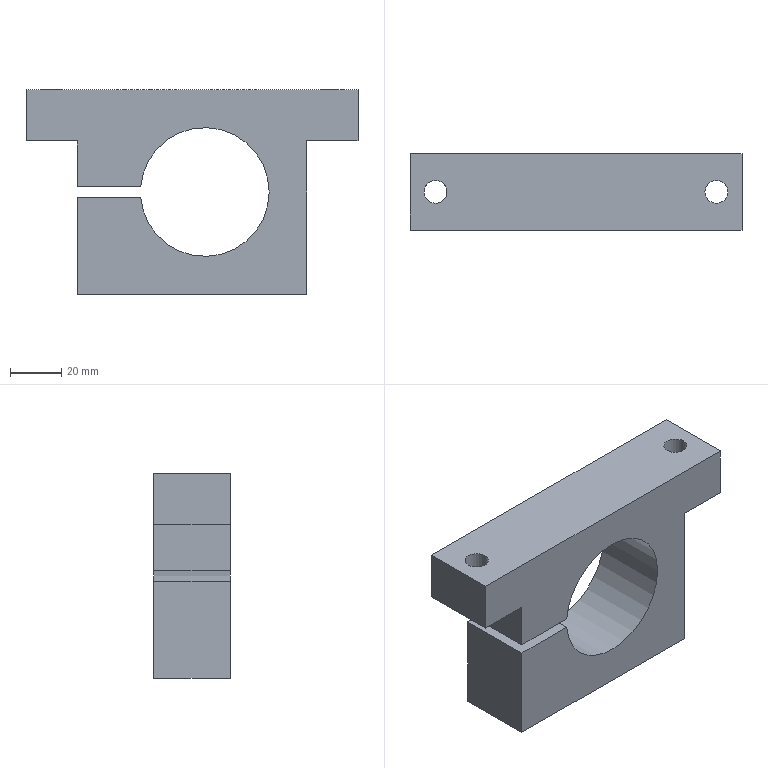Part | NX | features MAIN_BODY 2 | 1 solid | 16 faces | box 130 x 30 x 80 mm | volume 174625 mm3 | plane 13 | cylinder 3 | commonest cylinder face diameters 9 x2 50.4 x1
STEP:
#1=CARTESIAN_POINT('',(-547.,-675.001,150.));
#2=VERTEX_POINT('',#1);
#3=CARTESIAN_POINT('',(-547.,-675.001,170.));
#4=VERTEX_POINT('',#3);
#5=CARTESIAN_POINT('',(-547.,-675.001,150.));
#6=DIRECTION('',(0.,0.,1.));
#7=VECTOR('',#6,1000.);
#8=LINE('',#5,#7);
#9=EDGE_CURVE('',#2,#4,#8,.T.);
#10=ORIENTED_EDGE('',*,*,#9,.F.);
#11=CARTESIAN_POINT('',(-547.,-705.001,150.));
#12=VERTEX_POINT('',#11);
#13=CARTESIAN_POINT('',(-547.,-705.001,150.));
#14=DIRECTION('',(0.,1.,0.));
#15=VECTOR('',#14,1000.);
#16=LINE('',#13,#15);
#17=EDGE_CURVE('',#12,#2,#16,.T.);
#18=ORIENTED_EDGE('',*,*,#17,.F.);
#19=CARTESIAN_POINT('',(-547.,-705.001,170.));
#20=VERTEX_POINT('',#19);
#21=CARTESIAN_POINT('',(-547.,-705.001,150.));
#22=DIRECTION('',(0.,0.,1.));
#23=VECTOR('',#22,1000.);
#24=LINE('',#21,#23);
#25=EDGE_CURVE('',#12,#20,#24,.T.);
#26=ORIENTED_EDGE('',*,*,#25,.T.);
#27=CARTESIAN_POINT('',(-547.,-705.001,170.));
#28=DIRECTION('',(0.,1.,0.));
#29=VECTOR('',#28,1000.);
#30=LINE('',#27,#29);
#31=EDGE_CURVE('',#20,#4,#30,.T.);
#32=ORIENTED_EDGE('',*,*,#31,.T.);
#33=EDGE_LOOP('',(#10,#18,#26,#32));
#34=FACE_BOUND('',#33,.T.);
#35=CARTESIAN_POINT('',(-547.,-705.001,150.));
#36=DIRECTION('',(-1.,0.,0.));
#37=DIRECTION('',(0.,1.,0.));
#38=AXIS2_PLACEMENT_3D('',#35,#36,#37);
#39=PLANE('',#38);
#40=ADVANCED_FACE('',(#34),#39,.T.);
#41=CARTESIAN_POINT('',(-431.5,-690.001,170.));
#42=VERTEX_POINT('',#41);
#43=CARTESIAN_POINT('',(-427.,-690.001,170.));
#44=DIRECTION('',(0.,0.,1.));
#45=DIRECTION('',(-1.,0.,0.));
#46=AXIS2_PLACEMENT_3D('',#43,#44,#45);
#47=CIRCLE('',#46,4.5);
#48=EDGE_CURVE('',#42,#42,#47,.T.);
#49=ORIENTED_EDGE('',*,*,#48,.F.);
#50=EDGE_LOOP('',(#49));
#51=FACE_BOUND('',#50,.T.);
#52=CARTESIAN_POINT('',(-541.5,-690.001,170.));
#53=VERTEX_POINT('',#52);
#54=CARTESIAN_POINT('',(-537.,-690.001,170.));
#55=DIRECTION('',(0.,0.,1.));
#56=DIRECTION('',(-1.,0.,0.));
#57=AXIS2_PLACEMENT_3D('',#54,#55,#56);
#58=CIRCLE('',#57,4.5);
#59=EDGE_CURVE('',#53,#53,#58,.T.);
#60=ORIENTED_EDGE('',*,*,#59,.F.);
#61=EDGE_LOOP('',(#60));
#62=FACE_BOUND('',#61,.T.);
#63=CARTESIAN_POINT('',(-417.,-675.001,170.));
#64=VERTEX_POINT('',#63);
#65=CARTESIAN_POINT('',(-547.,-675.001,170.));
#66=DIRECTION('',(1.,0.,0.));
#67=VECTOR('',#66,1000.);
#68=LINE('',#65,#67);
#69=EDGE_CURVE('',#4,#64,#68,.T.);
#70=ORIENTED_EDGE('',*,*,#69,.F.);
#71=ORIENTED_EDGE('',*,*,#31,.F.);
#72=CARTESIAN_POINT('',(-417.,-705.001,170.));
#73=VERTEX_POINT('',#72);
#74=CARTESIAN_POINT('',(-547.,-705.001,170.));
#75=DIRECTION('',(1.,0.,0.));
#76=VECTOR('',#75,1000.);
#77=LINE('',#74,#76);
#78=EDGE_CURVE('',#20,#73,#77,.T.);
#79=ORIENTED_EDGE('',*,*,#78,.T.);
#80=CARTESIAN_POINT('',(-417.,-705.001,170.));
#81=DIRECTION('',(0.,1.,0.));
#82=VECTOR('',#81,1000.);
#83=LINE('',#80,#82);
#84=EDGE_CURVE('',#73,#64,#83,.T.);
#85=ORIENTED_EDGE('',*,*,#84,.T.);
#86=EDGE_LOOP('',(#70,#71,#79,#85));
#87=FACE_BOUND('',#86,.T.);
#88=CARTESIAN_POINT('',(-547.,-705.001,170.));
#89=DIRECTION('',(0.,0.,1.));
#90=DIRECTION('',(-1.,0.,0.));
#91=AXIS2_PLACEMENT_3D('',#88,#89,#90);
#92=PLANE('',#91);
#93=ADVANCED_FACE('',(#51,#62,#87),#92,.T.);
#94=CARTESIAN_POINT('',(-417.,-675.001,150.));
#95=VERTEX_POINT('',#94);
#96=CARTESIAN_POINT('',(-417.,-675.001,170.));
#97=DIRECTION('',(0.,0.,-1.));
#98=VECTOR('',#97,1000.);
#99=LINE('',#96,#98);
#100=EDGE_CURVE('',#64,#95,#99,.T.);
#101=ORIENTED_EDGE('',*,*,#100,.F.);
#102=ORIENTED_EDGE('',*,*,#84,.F.);
#103=CARTESIAN_POINT('',(-417.,-705.001,150.));
#104=VERTEX_POINT('',#103);
#105=CARTESIAN_POINT('',(-417.,-705.001,170.));
#106=DIRECTION('',(0.,0.,-1.));
#107=VECTOR('',#106,1000.);
#108=LINE('',#105,#107);
#109=EDGE_CURVE('',#73,#104,#108,.T.);
#110=ORIENTED_EDGE('',*,*,#109,.T.);
#111=CARTESIAN_POINT('',(-417.,-705.001,150.));
#112=DIRECTION('',(0.,1.,0.));
#113=VECTOR('',#112,1000.);
#114=LINE('',#111,#113);
#115=EDGE_CURVE('',#104,#95,#114,.T.);
#116=ORIENTED_EDGE('',*,*,#115,.T.);
#117=EDGE_LOOP('',(#101,#102,#110,#116));
#118=FACE_BOUND('',#117,.T.);
#119=CARTESIAN_POINT('',(-417.,-705.001,170.));
#120=DIRECTION('',(1.,0.,0.));
#121=DIRECTION('',(0.,0.,1.));
#122=AXIS2_PLACEMENT_3D('',#119,#120,#121);
#123=PLANE('',#122);
#124=ADVANCED_FACE('',(#118),#123,.T.);
#125=CARTESIAN_POINT('',(-431.5,-690.001,150.));
#126=VERTEX_POINT('',#125);
#127=CARTESIAN_POINT('',(-427.,-690.001,150.));
#128=DIRECTION('',(0.,0.,1.));
#129=DIRECTION('',(-1.,0.,0.));
#130=AXIS2_PLACEMENT_3D('',#127,#128,#129);
#131=CIRCLE('',#130,4.5);
#132=EDGE_CURVE('',#126,#126,#131,.T.);
#133=ORIENTED_EDGE('',*,*,#132,.T.);
#134=EDGE_LOOP('',(#133));
#135=FACE_BOUND('',#134,.T.);
#136=CARTESIAN_POINT('',(-437.,-675.001,150.));
#137=VERTEX_POINT('',#136);
#138=CARTESIAN_POINT('',(-437.,-675.001,150.));
#139=DIRECTION('',(1.,0.,0.));
#140=VECTOR('',#139,1000.);
#141=LINE('',#138,#140);
#142=EDGE_CURVE('',#137,#95,#141,.T.);
#143=ORIENTED_EDGE('',*,*,#142,.T.);
#144=ORIENTED_EDGE('',*,*,#115,.F.);
#145=CARTESIAN_POINT('',(-437.,-705.001,150.));
#146=VERTEX_POINT('',#145);
#147=CARTESIAN_POINT('',(-437.,-705.001,150.));
#148=DIRECTION('',(1.,0.,0.));
#149=VECTOR('',#148,1000.);
#150=LINE('',#147,#149);
#151=EDGE_CURVE('',#146,#104,#150,.T.);
#152=ORIENTED_EDGE('',*,*,#151,.F.);
#153=CARTESIAN_POINT('',(-437.,-705.001,150.));
#154=DIRECTION('',(0.,1.,0.));
#155=VECTOR('',#154,1000.);
#156=LINE('',#153,#155);
#157=EDGE_CURVE('',#146,#137,#156,.T.);
#158=ORIENTED_EDGE('',*,*,#157,.T.);
#159=EDGE_LOOP('',(#143,#144,#152,#158));
#160=FACE_BOUND('',#159,.T.);
#161=CARTESIAN_POINT('',(-437.,-705.001,150.));
#162=DIRECTION('',(0.,0.,1.));
#163=DIRECTION('',(-1.,0.,0.));
#164=AXIS2_PLACEMENT_3D('',#161,#162,#163);
#165=PLANE('',#164);
#166=ADVANCED_FACE('',(#135,#160),#165,.F.);
#167=CARTESIAN_POINT('',(-437.,-675.001,90.));
#168=VERTEX_POINT('',#167);
#169=CARTESIAN_POINT('',(-437.,-675.001,90.));
#170=DIRECTION('',(0.,0.,1.));
#171=VECTOR('',#170,1000.);
#172=LINE('',#169,#171);
#173=EDGE_CURVE('',#168,#137,#172,.T.);
#174=ORIENTED_EDGE('',*,*,#173,.T.);
#175=ORIENTED_EDGE('',*,*,#157,.F.);
#176=CARTESIAN_POINT('',(-437.,-705.001,90.));
#177=VERTEX_POINT('',#176);
#178=CARTESIAN_POINT('',(-437.,-705.001,90.));
#179=DIRECTION('',(0.,0.,1.));
#180=VECTOR('',#179,1000.);
#181=LINE('',#178,#180);
#182=EDGE_CURVE('',#177,#146,#181,.T.);
#183=ORIENTED_EDGE('',*,*,#182,.F.);
#184=CARTESIAN_POINT('',(-437.,-705.001,90.));
#185=DIRECTION('',(0.,1.,0.));
#186=VECTOR('',#185,1000.);
#187=LINE('',#184,#186);
#188=EDGE_CURVE('',#177,#168,#187,.T.);
#189=ORIENTED_EDGE('',*,*,#188,.T.);
#190=EDGE_LOOP('',(#174,#175,#183,#189));
#191=FACE_BOUND('',#190,.T.);
#192=CARTESIAN_POINT('',(-437.,-705.001,90.));
#193=DIRECTION('',(-1.,0.,0.));
#194=DIRECTION('',(0.,0.,-1.));
#195=AXIS2_PLACEMENT_3D('',#192,#193,#194);
#196=PLANE('',#195);
#197=ADVANCED_FACE('',(#191),#196,.F.);
#198=CARTESIAN_POINT('',(-527.,-675.001,90.));
#199=VERTEX_POINT('',#198);
#200=CARTESIAN_POINT('',(-437.,-675.001,90.));
#201=DIRECTION('',(-1.,0.,0.));
#202=VECTOR('',#201,1000.);
#203=LINE('',#200,#202);
#204=EDGE_CURVE('',#168,#199,#203,.T.);
#205=ORIENTED_EDGE('',*,*,#204,.F.);
#206=ORIENTED_EDGE('',*,*,#188,.F.);
#207=CARTESIAN_POINT('',(-527.,-705.001,90.));
#208=VERTEX_POINT('',#207);
#209=CARTESIAN_POINT('',(-437.,-705.001,90.));
#210=DIRECTION('',(-1.,0.,0.));
#211=VECTOR('',#210,1000.);
#212=LINE('',#209,#211);
#213=EDGE_CURVE('',#177,#208,#212,.T.);
#214=ORIENTED_EDGE('',*,*,#213,.T.);
#215=CARTESIAN_POINT('',(-527.,-705.001,90.));
#216=DIRECTION('',(0.,1.,0.));
#217=VECTOR('',#216,1000.);
#218=LINE('',#215,#217);
#219=EDGE_CURVE('',#208,#199,#218,.T.);
#220=ORIENTED_EDGE('',*,*,#219,.T.);
#221=EDGE_LOOP('',(#205,#206,#214,#220));
#222=FACE_BOUND('',#221,.T.);
#223=CARTESIAN_POINT('',(-437.,-705.001,90.));
#224=DIRECTION('',(0.,0.,-1.));
#225=DIRECTION('',(0.,-1.,0.));
#226=AXIS2_PLACEMENT_3D('',#223,#224,#225);
#227=PLANE('',#226);
#228=ADVANCED_FACE('',(#222),#227,.T.);
#229=CARTESIAN_POINT('',(-527.,-675.001,128.));
#230=VERTEX_POINT('',#229);
#231=CARTESIAN_POINT('',(-527.,-675.001,90.));
#232=DIRECTION('',(0.,0.,1.));
#233=VECTOR('',#232,1000.);
#234=LINE('',#231,#233);
#235=EDGE_CURVE('',#199,#230,#234,.T.);
#236=ORIENTED_EDGE('',*,*,#235,.F.);
#237=ORIENTED_EDGE('',*,*,#219,.F.);
#238=CARTESIAN_POINT('',(-527.,-705.001,128.));
#239=VERTEX_POINT('',#238);
#240=CARTESIAN_POINT('',(-527.,-705.001,90.));
#241=DIRECTION('',(0.,0.,1.));
#242=VECTOR('',#241,1000.);
#243=LINE('',#240,#242);
#244=EDGE_CURVE('',#208,#239,#243,.T.);
#245=ORIENTED_EDGE('',*,*,#244,.T.);
#246=CARTESIAN_POINT('',(-527.,-705.001,128.));
#247=DIRECTION('',(0.,1.,0.));
#248=VECTOR('',#247,1000.);
#249=LINE('',#246,#248);
#250=EDGE_CURVE('',#239,#230,#249,.T.);
#251=ORIENTED_EDGE('',*,*,#250,.T.);
#252=EDGE_LOOP('',(#236,#237,#245,#251));
#253=FACE_BOUND('',#252,.T.);
#254=CARTESIAN_POINT('',(-527.,-705.001,90.));
#255=DIRECTION('',(-1.,0.,0.));
#256=DIRECTION('',(0.,1.,0.));
#257=AXIS2_PLACEMENT_3D('',#254,#255,#256);
#258=PLANE('',#257);
#259=ADVANCED_FACE('',(#253),#258,.T.);
#260=CARTESIAN_POINT('',(-502.121,-675.001,128.));
#261=VERTEX_POINT('',#260);
#262=CARTESIAN_POINT('',(-502.121,-675.001,128.));
#263=DIRECTION('',(-1.,0.,0.));
#264=VECTOR('',#263,1000.);
#265=LINE('',#262,#264);
#266=EDGE_CURVE('',#261,#230,#265,.T.);
#267=ORIENTED_EDGE('',*,*,#266,.T.);
#268=ORIENTED_EDGE('',*,*,#250,.F.);
#269=CARTESIAN_POINT('',(-502.121,-705.001,128.));
#270=VERTEX_POINT('',#269);
#271=CARTESIAN_POINT('',(-502.121,-705.001,128.));
#272=DIRECTION('',(-1.,0.,0.));
#273=VECTOR('',#272,1000.);
#274=LINE('',#271,#273);
#275=EDGE_CURVE('',#270,#239,#274,.T.);
#276=ORIENTED_EDGE('',*,*,#275,.F.);
#277=CARTESIAN_POINT('',(-502.121,-705.001,128.));
#278=DIRECTION('',(0.,1.,0.));
#279=VECTOR('',#278,1000.);
#280=LINE('',#277,#279);
#281=EDGE_CURVE('',#270,#261,#280,.T.);
#282=ORIENTED_EDGE('',*,*,#281,.T.);
#283=EDGE_LOOP('',(#267,#268,#276,#282));
#284=FACE_BOUND('',#283,.T.);
#285=CARTESIAN_POINT('',(-502.121,-705.001,128.));
#286=DIRECTION('',(0.,0.,-1.));
#287=DIRECTION('',(1.,0.,0.));
#288=AXIS2_PLACEMENT_3D('',#285,#286,#287);
#289=PLANE('',#288);
#290=ADVANCED_FACE('',(#284),#289,.F.);
#291=CARTESIAN_POINT('',(-502.121,-675.001,132.));
#292=VERTEX_POINT('',#291);
#293=CARTESIAN_POINT('',(-477.,-675.001,130.));
#294=DIRECTION('',(0.,-1.,0.));
#295=DIRECTION('',(-1.,0.,0.));
#296=AXIS2_PLACEMENT_3D('',#293,#294,#295);
#297=CIRCLE('',#296,25.2);
#298=EDGE_CURVE('',#261,#292,#297,.T.);
#299=ORIENTED_EDGE('',*,*,#298,.F.);
#300=ORIENTED_EDGE('',*,*,#281,.F.);
#301=CARTESIAN_POINT('',(-502.121,-705.001,132.));
#302=VERTEX_POINT('',#301);
#303=CARTESIAN_POINT('',(-477.,-705.001,130.));
#304=DIRECTION('',(0.,-1.,0.));
#305=DIRECTION('',(-1.,0.,0.));
#306=AXIS2_PLACEMENT_3D('',#303,#304,#305);
#307=CIRCLE('',#306,25.2);
#308=EDGE_CURVE('',#270,#302,#307,.T.);
#309=ORIENTED_EDGE('',*,*,#308,.T.);
#310=CARTESIAN_POINT('',(-502.121,-705.001,132.));
#311=DIRECTION('',(0.,1.,0.));
#312=VECTOR('',#311,1000.);
#313=LINE('',#310,#312);
#314=EDGE_CURVE('',#302,#292,#313,.T.);
#315=ORIENTED_EDGE('',*,*,#314,.T.);
#316=EDGE_LOOP('',(#299,#300,#309,#315));
#317=FACE_BOUND('',#316,.T.);
#318=CARTESIAN_POINT('',(-477.,-705.001,130.));
#319=DIRECTION('',(0.,1.,0.));
#320=DIRECTION('',(1.,0.,0.));
#321=AXIS2_PLACEMENT_3D('',#318,#319,#320);
#322=CYLINDRICAL_SURFACE('',#321,25.2);
#323=ADVANCED_FACE('',(#317),#322,.F.);
#324=CARTESIAN_POINT('',(-527.,-675.001,132.));
#325=VERTEX_POINT('',#324);
#326=CARTESIAN_POINT('',(-502.121,-675.001,132.));
#327=DIRECTION('',(-1.,0.,0.));
#328=VECTOR('',#327,1000.);
#329=LINE('',#326,#328);
#330=EDGE_CURVE('',#292,#325,#329,.T.);
#331=ORIENTED_EDGE('',*,*,#330,.F.);
#332=ORIENTED_EDGE('',*,*,#314,.F.);
#333=CARTESIAN_POINT('',(-527.,-705.001,132.));
#334=VERTEX_POINT('',#333);
#335=CARTESIAN_POINT('',(-502.121,-705.001,132.));
#336=DIRECTION('',(-1.,0.,0.));
#337=VECTOR('',#336,1000.);
#338=LINE('',#335,#337);
#339=EDGE_CURVE('',#302,#334,#338,.T.);
#340=ORIENTED_EDGE('',*,*,#339,.T.);
#341=CARTESIAN_POINT('',(-527.,-705.001,132.));
#342=DIRECTION('',(0.,1.,0.));
#343=VECTOR('',#342,1000.);
#344=LINE('',#341,#343);
#345=EDGE_CURVE('',#334,#325,#344,.T.);
#346=ORIENTED_EDGE('',*,*,#345,.T.);
#347=EDGE_LOOP('',(#331,#332,#340,#346));
#348=FACE_BOUND('',#347,.T.);
#349=CARTESIAN_POINT('',(-502.121,-705.001,132.));
#350=DIRECTION('',(0.,0.,-1.));
#351=DIRECTION('',(1.,0.,0.));
#352=AXIS2_PLACEMENT_3D('',#349,#350,#351);
#353=PLANE('',#352);
#354=ADVANCED_FACE('',(#348),#353,.T.);
#355=CARTESIAN_POINT('',(-527.,-675.001,150.));
#356=VERTEX_POINT('',#355);
#357=CARTESIAN_POINT('',(-527.,-675.001,132.));
#358=DIRECTION('',(0.,0.,1.));
#359=VECTOR('',#358,1000.);
#360=LINE('',#357,#359);
#361=EDGE_CURVE('',#325,#356,#360,.T.);
#362=ORIENTED_EDGE('',*,*,#361,.F.);
#363=ORIENTED_EDGE('',*,*,#345,.F.);
#364=CARTESIAN_POINT('',(-527.,-705.001,150.));
#365=VERTEX_POINT('',#364);
#366=CARTESIAN_POINT('',(-527.,-705.001,132.));
#367=DIRECTION('',(0.,0.,1.));
#368=VECTOR('',#367,1000.);
#369=LINE('',#366,#368);
#370=EDGE_CURVE('',#334,#365,#369,.T.);
#371=ORIENTED_EDGE('',*,*,#370,.T.);
#372=CARTESIAN_POINT('',(-527.,-705.001,150.));
#373=DIRECTION('',(0.,1.,0.));
#374=VECTOR('',#373,1000.);
#375=LINE('',#372,#374);
#376=EDGE_CURVE('',#365,#356,#375,.T.);
#377=ORIENTED_EDGE('',*,*,#376,.T.);
#378=EDGE_LOOP('',(#362,#363,#371,#377));
#379=FACE_BOUND('',#378,.T.);
#380=CARTESIAN_POINT('',(-527.,-705.001,132.));
#381=DIRECTION('',(-1.,0.,0.));
#382=DIRECTION('',(0.,1.,0.));
#383=AXIS2_PLACEMENT_3D('',#380,#381,#382);
#384=PLANE('',#383);
#385=ADVANCED_FACE('',(#379),#384,.T.);
#386=CARTESIAN_POINT('',(-537.,-685.501,150.));
#387=VERTEX_POINT('',#386);
#388=CARTESIAN_POINT('',(-537.,-690.001,150.));
#389=DIRECTION('',(0.,0.,1.));
#390=DIRECTION('',(0.,1.,0.));
#391=AXIS2_PLACEMENT_3D('',#388,#389,#390);
#392=CIRCLE('',#391,4.5);
#393=EDGE_CURVE('',#387,#387,#392,.T.);
#394=ORIENTED_EDGE('',*,*,#393,.T.);
#395=EDGE_LOOP('',(#394));
#396=FACE_BOUND('',#395,.T.);
#397=CARTESIAN_POINT('',(-527.,-675.001,150.));
#398=DIRECTION('',(-1.,0.,0.));
#399=VECTOR('',#398,1000.);
#400=LINE('',#397,#399);
#401=EDGE_CURVE('',#356,#2,#400,.T.);
#402=ORIENTED_EDGE('',*,*,#401,.F.);
#403=ORIENTED_EDGE('',*,*,#376,.F.);
#404=CARTESIAN_POINT('',(-527.,-705.001,150.));
#405=DIRECTION('',(-1.,0.,0.));
#406=VECTOR('',#405,1000.);
#407=LINE('',#404,#406);
#408=EDGE_CURVE('',#365,#12,#407,.T.);
#409=ORIENTED_EDGE('',*,*,#408,.T.);
#410=ORIENTED_EDGE('',*,*,#17,.T.);
#411=EDGE_LOOP('',(#402,#403,#409,#410));
#412=FACE_BOUND('',#411,.T.);
#413=CARTESIAN_POINT('',(-527.,-705.001,150.));
#414=DIRECTION('',(0.,0.,-1.));
#415=DIRECTION('',(0.,-1.,0.));
#416=AXIS2_PLACEMENT_3D('',#413,#414,#415);
#417=PLANE('',#416);
#418=ADVANCED_FACE('',(#396,#412),#417,.T.);
#419=ORIENTED_EDGE('',*,*,#25,.F.);
#420=ORIENTED_EDGE('',*,*,#408,.F.);
#421=ORIENTED_EDGE('',*,*,#370,.F.);
#422=ORIENTED_EDGE('',*,*,#339,.F.);
#423=ORIENTED_EDGE('',*,*,#308,.F.);
#424=ORIENTED_EDGE('',*,*,#275,.T.);
#425=ORIENTED_EDGE('',*,*,#244,.F.);
#426=ORIENTED_EDGE('',*,*,#213,.F.);
#427=ORIENTED_EDGE('',*,*,#182,.T.);
#428=ORIENTED_EDGE('',*,*,#151,.T.);
#429=ORIENTED_EDGE('',*,*,#109,.F.);
#430=ORIENTED_EDGE('',*,*,#78,.F.);
#431=EDGE_LOOP('',(#419,#420,#421,#422,#423,#424,#425,#426,#427,#428,#429,#430));
#432=FACE_BOUND('',#431,.T.);
#433=CARTESIAN_POINT('',(-477.,-705.001,130.));
#434=DIRECTION('',(0.,-1.,0.));
#435=DIRECTION('',(-1.,0.,0.));
#436=AXIS2_PLACEMENT_3D('',#433,#434,#435);
#437=PLANE('',#436);
#438=ADVANCED_FACE('',(#432),#437,.T.);
#439=ORIENTED_EDGE('',*,*,#9,.T.);
#440=ORIENTED_EDGE('',*,*,#69,.T.);
#441=ORIENTED_EDGE('',*,*,#100,.T.);
#442=ORIENTED_EDGE('',*,*,#142,.F.);
#443=ORIENTED_EDGE('',*,*,#173,.F.);
#444=ORIENTED_EDGE('',*,*,#204,.T.);
#445=ORIENTED_EDGE('',*,*,#235,.T.);
#446=ORIENTED_EDGE('',*,*,#266,.F.);
#447=ORIENTED_EDGE('',*,*,#298,.T.);
#448=ORIENTED_EDGE('',*,*,#330,.T.);
#449=ORIENTED_EDGE('',*,*,#361,.T.);
#450=ORIENTED_EDGE('',*,*,#401,.T.);
#451=EDGE_LOOP('',(#439,#440,#441,#442,#443,#444,#445,#446,#447,#448,#449,#450));
#452=FACE_BOUND('',#451,.T.);
#453=CARTESIAN_POINT('',(-477.,-675.001,130.));
#454=DIRECTION('',(0.,-1.,0.));
#455=DIRECTION('',(-1.,0.,0.));
#456=AXIS2_PLACEMENT_3D('',#453,#454,#455);
#457=PLANE('',#456);
#458=ADVANCED_FACE('',(#452),#457,.F.);
#459=ORIENTED_EDGE('',*,*,#59,.T.);
#460=EDGE_LOOP('',(#459));
#461=FACE_BOUND('',#460,.T.);
#462=ORIENTED_EDGE('',*,*,#393,.F.);
#463=EDGE_LOOP('',(#462));
#464=FACE_BOUND('',#463,.T.);
#465=CARTESIAN_POINT('',(-537.,-690.001,150.));
#466=DIRECTION('',(0.,0.,1.));
#467=DIRECTION('',(0.,1.,0.));
#468=AXIS2_PLACEMENT_3D('',#465,#466,#467);
#469=CYLINDRICAL_SURFACE('',#468,4.5);
#470=ADVANCED_FACE('',(#461,#464),#469,.F.);
#471=ORIENTED_EDGE('',*,*,#48,.T.);
#472=EDGE_LOOP('',(#471));
#473=FACE_BOUND('',#472,.T.);
#474=ORIENTED_EDGE('',*,*,#132,.F.);
#475=EDGE_LOOP('',(#474));
#476=FACE_BOUND('',#475,.T.);
#477=CARTESIAN_POINT('',(-427.,-690.001,150.));
#478=DIRECTION('',(0.,0.,1.));
#479=DIRECTION('',(-1.,0.,0.));
#480=AXIS2_PLACEMENT_3D('',#477,#478,#479);
#481=CYLINDRICAL_SURFACE('',#480,4.5);
#482=ADVANCED_FACE('',(#473,#476),#481,.F.);
#483=CLOSED_SHELL('',(#40,#93,#124,#166,#197,#228,#259,#290,#323,#354,#385,#418,#438,#458,#470,#482));
#484=MANIFOLD_SOLID_BREP('',#483);
#485=(LENGTH_UNIT()NAMED_UNIT(*)SI_UNIT(.MILLI.,.METRE.));
#486=UNCERTAINTY_MEASURE_WITH_UNIT(LENGTH_MEASURE(0.00001),#485,'','');
#487=(NAMED_UNIT(*)PLANE_ANGLE_UNIT()SI_UNIT($,.RADIAN.));
#488=(NAMED_UNIT(*)SI_UNIT($,.STERADIAN.)SOLID_ANGLE_UNIT());
#489=(GEOMETRIC_REPRESENTATION_CONTEXT(3)GLOBAL_UNCERTAINTY_ASSIGNED_CONTEXT((#486))GLOBAL_UNIT_ASSIGNED_CONTEXT((#485,#487,#488))REPRESENTATION_CONTEXT('',''));
#490=ADVANCED_BREP_SHAPE_REPRESENTATION('',(#484),#489);